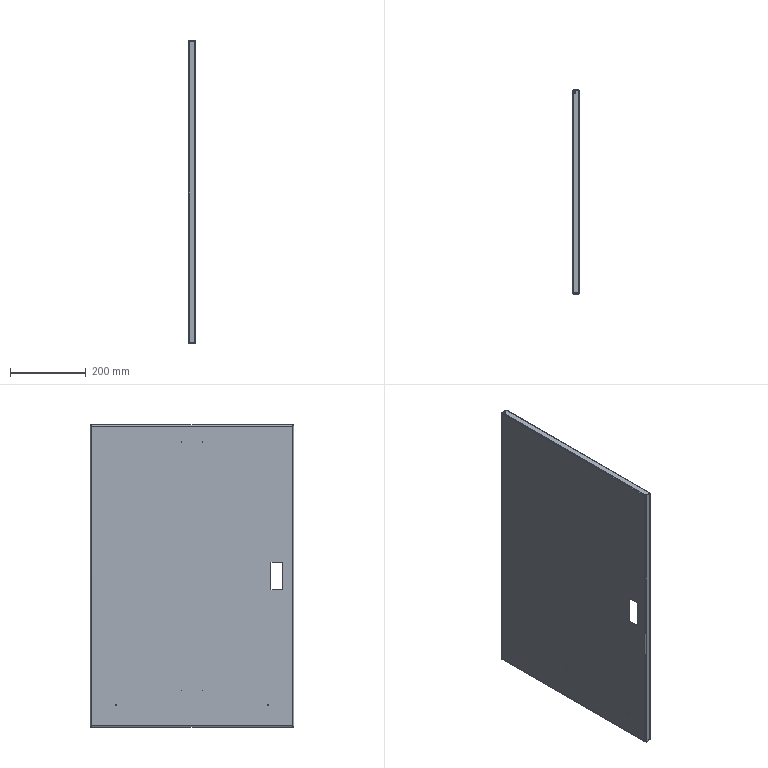Part | NX | features solid 2 | 1 solid | 143 faces | box 20 x 536 x 796 mm | volume 753874 mm3 | plane 76 | cylinder 36 | spline 31 | commonest cylinder face diameters 1 x12 6 x12 3 x8 7 x4